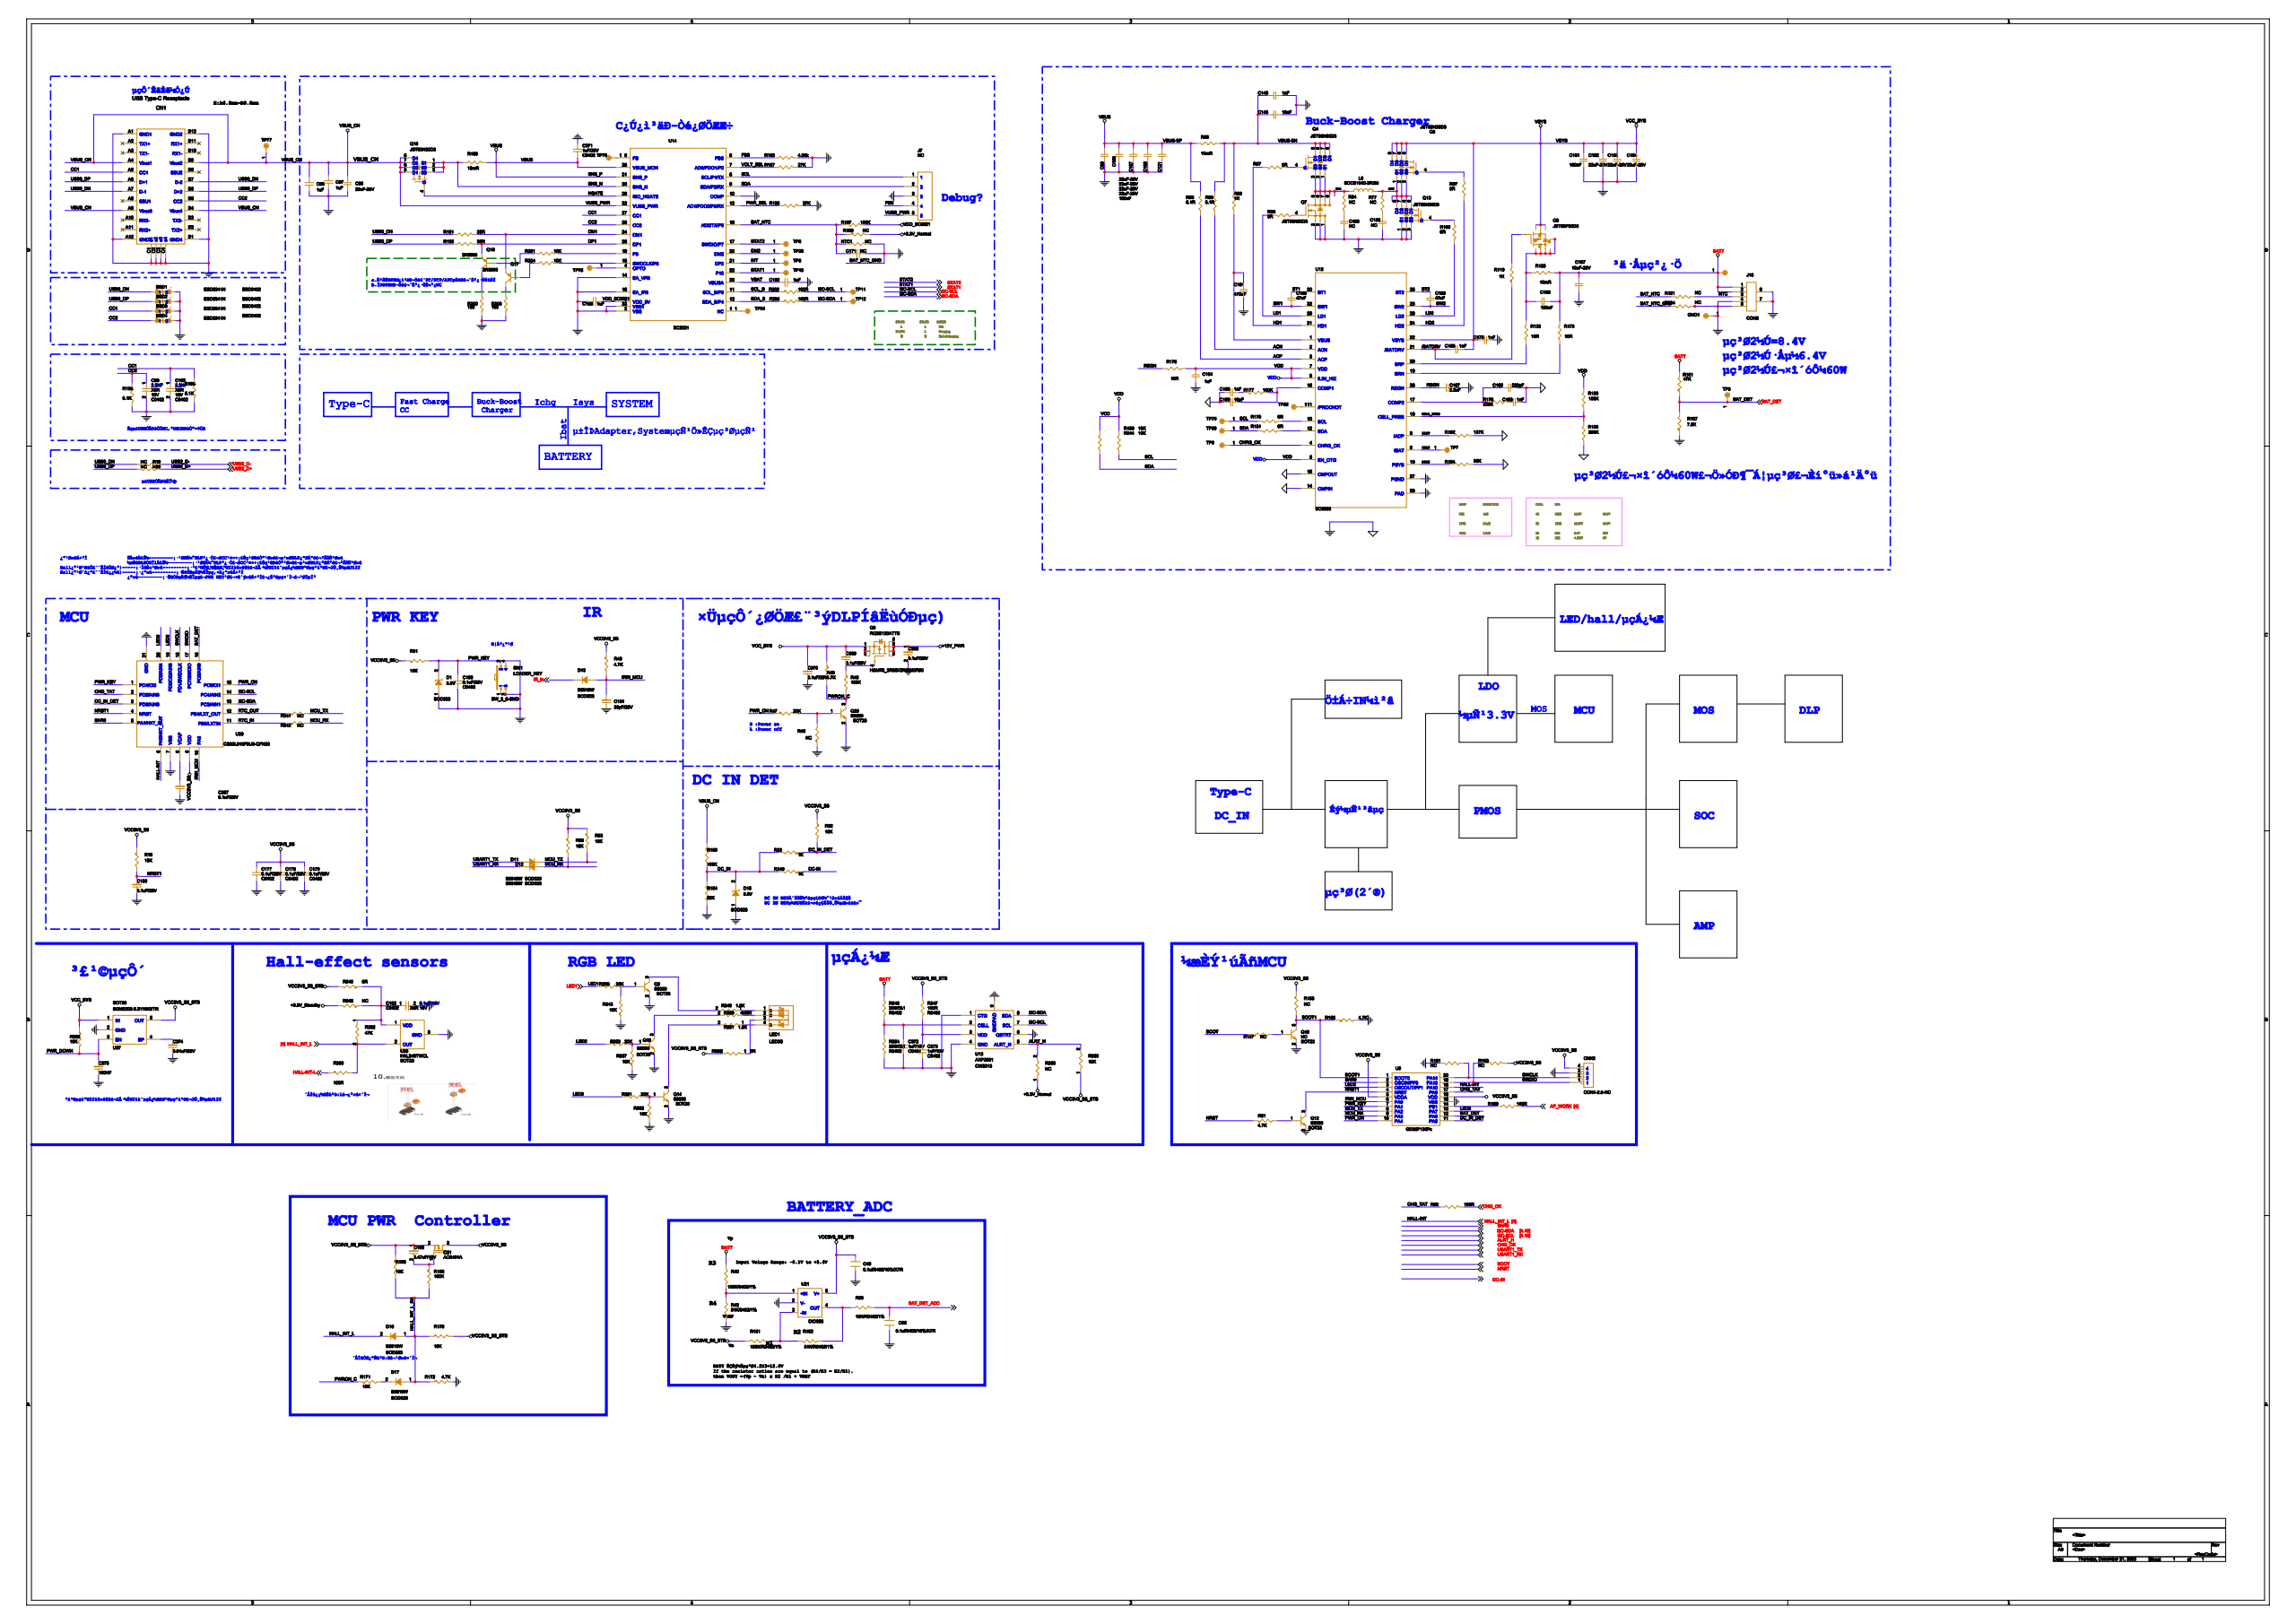Circuit board | Cadence Allegro | 1223 parts | 777 nets | one sheet of the schematic
Parts on this sheet (reference | value | footprint):
C49 | 0.1uf/0402/10%/X7R | C0402
C85 | 0.1uf/0402/10%/X7R | C0402
C95 | 22uF-25V | C1206
C96 | 22uF-25V | C1206
C97 | 1uF | C0402
C98 | 1uF | C0402
C99 | 2.2NF | C0402
C102 | 2.2NF | C0402
C108 | 22uF-25V | C1206
C121 | 100nF | C0402
C148 | 10nF | C0402
C149 | 1nF | C0402
C150 | 22uF-25V | C1206
C151 | 100nF | C0402
C152 | 22uF-25V | C1206
C153 | 22uF-25V | C1206
C154 | 22uF-25V | C1206
C155 | NC | C0402
C156 | NC | C0402
C157 | 10uF-25V | C0805
C158 | 47nF | C0402
C159 | 47nF | C0402
C160 | 100nF | C0402
C161 | 470nF | C0402
C162 | 0.1uF/16V | C0402
C163 | 1nF | C0402
C164 | 1uF | C0402
C165 | 220pF | C0402
C166 | 1nF | C0402
C167 | 2.2uF | C0402
C168 | 1nF | C0402
C169 | 10pF | C0402
C171 | NC | C0402
C175 | 1uF | C0402
C177 | 0.1uF/25V | C0402
C178 | 0.1uF/25V | C0402
C179 | 0.1uF/25V | C0402
C180 | 0.1uF/25V | C0402
C181 | 33pF/25V | C0402
C192 | 1uF | C0402
C193 | 1uF | C0402
C195 | 0.47uF/16V | C0402
C196 | 0.1uF/25V | C0402
C367 | 0.1uF/25V | C0402
C368 | 0.1uF/25V | C0402
C369 | 0.1uF/25V | C0402
C370 | 0.1uF/25V | C0402
C371 | 1uF/25V | C0402
C372 | 1uF/10V | C0402
C373 | 1uF/10V | C0402
C374 | 0.01uF/25V | C0402
C375 | 100NF | C0402
CN1 | USB Type-C Receptacle | USB_TYPE_C
CNX2 | CON4-2.0-NC | DIP4PIN-2P0MM
D1 | 3.3V | SOD323
D11 | B5819W | SOD323
D12 | B5819W | SOD323
D13 | B5819W | SOD323
D15 | 3.3V | SOD323
D16 | B5819W | SOD323
D17 | B5819W | SOD323
ESD1 | ESD5341N | ESD0402
ESD2 | ESD5341N | ESD0402
ESD3 | ESD5341N | ESD0402
ESD4 | ESD5341N | ESD0402
GND2 | DEO | TP06MM
J7 | NC | SIP5P
J10 | CON5 | CN1X5-1P25MM-WF
L6 | SCCB1040-2R2M | L1040
LED1 | LED3S | DIP4PIN-1P25MM
NTC1 | NC | R0603
Q3 | RQ3E120ATTB | HSMT8_3R30X3R30X0R90
Q4 | JST60N30D3 | HSMT8_3R30X3R30X0R90
Q5 | JST60P30D5 | DFN8
Q6 | JST60N30D3 | HSMT8_3R30X3R30X0R90
Q7 | JST60N30D3 | HSMT8_3R30X3R30X0R90
Q9 | S8050 | SOT23
Q10 | S8050 | SOT23
Q12 | S8050 | SOT23
Q13 | JST60N30D3 | HSMT8_3R30X3R30X0R90
Q14 | S8050 | SOT23
Q15 | JST60N30D3 | HSMT8_3R30X3R30X0R90
Q16 | 2N3906 | SOT-23
Q17 | 2N3906 | SOT-23
Q18 | NC | SOT23
Q21 | AO3401A | SOT23-100
Q23 | S8050 | SOT23
R18 | 10K | R0402
R19 | NC | R0402
R20 | NC | R0402
R31 | 10K | R0402
R32 | 10K | R0402
R33 | 1K | R0402
R40 | 100K/0402/1% | R0402
R42 | 51K/0402/1% | R0402
R43 | 4.7K | R0402
R46 | 100K | R0402
R47 | 20K | R0402
R48 | NC | R0402
R49 | 4.7K | R0402
R50 | 100R | R0402
R51 | 4.7K | R0402
R53 | 10K | R0402
R56 | 10mR | R2010
R57 | 0R | R0402
R58 | 5.1R | R0402
R60 | 5.1R | R0402
R63 | 1R | R0402
R64 | NC | R0603
R77 | NC | R0603
R96 | 0R | R0402
R97 | 0R | R0402
R98 | 10K | R0402
R99 | 10K/R0402/1% | R0402
R100 | 0R | R0402
R101 | 47K | R0402
R107 | 7.5K | R0402
R119 | 1K | R0402
R120 | 10mR | R2010
R121 | NC | R0402
R122 | 10R | R0402
R149 | 1K | R0402
R150 | 100K | R0402
R152 | 51K/R0402/1% | R0402
R154 | 22K | R0402
R155 | NC | R0402
R156 | 4.7K | R0402
R157 | NC | R0402
R161 | NC | R0402
R163 | NC | R0402
R166 | 10K | R0402
R167 | 100K | R0402
R168 | 100K | R0402
R169 | 100R | R0402
R170 | 10K | R0402
R171 | 10K | R0402
R172 | 4.7K | R0402
R175 | 10R | R0402
R176 | 10R | R0603
R177 | 100K | R0402
R178 | 330K | R0402
R179 | 0R | R0402
R180 | 100K | R0402
R181 | 0R | R0402
R182 | 137K | R0402
R183 | 300K | R0402
R184 | 30K | R0402
R185 | 4.99k | R0402
R186 | 10mR | R2010
R187 | 27K | R0402
R188 | 27K | R0402
R189 | NC | R0402
R190 | 10K | R0603
R191 | 33R | R0402
R192 | 33R | R0402
R195 | 5.1K | R0402
R196 | 5.1K | R0402
R200 | 100 | R0402
R201 | 10K | R0402
R202 | 100R | R0402
R203 | 100 | R0402
R204 | 10K | R0402
R205 | 100R | R0402
R339 | 20K | R0402
R340 | 0R | R0402
R341 | NC | R0402
R342 | NC | R0402
R344 | 10K | R0603
R345 | 10K | R0402
R346 | 200K%1 | R0402
R347 | 100R | R0402
R348 | NC | R0402
R349 | 1.8K | R0402
R350 | 4.02K | R0402
R351 | 1.8K | R0402
R352 | 47K | R0402
R353 | 20K | R0402
R354 | 200K%1 | R0402
R355 | 10K | R0402
R357 | 10K | R0402
R358 | NC | R0402
R359 | 10K | R0402
R360 | 100R | R0402
R361 | 20K | R0402
R362 | 10K | R0402
R384 | NC | R0402
SW1 | LOADER_KEY | SW_3_6-SMD
TP5 | DEO | TP06MM
TP6 | DEO | TP06MM
TP7 | DEO | TP06MM
TP8 | DEO | TP06MM
TP9 | DEO | TP06MM
TP10 | DEO | TP06MM
TP11 | DEO | TP06MM
TP12 | DEO | TP06MM
TP26 | DEO | TP06MM
TP76 | DEO | TP06MM
TP77 | DEO | TP06MM
TP78 | DEO | TP06MM
TP79 | DEO | TP06MM
TP80 | DEO | TP06MM
TP81 | DEO | TP06MM
TP82 | DEO | TP06MM
U9 | GD32F130Fx | TSSOP20
U12 | SC8886 | QFN32_5X5MM
U13 | AXP2601 | CW2013
U14 | SC2021 | QFN32_5X5MM
U21 | DIO358 | SOT25
U37 | SGM2202-3.3YN5G/TR | SOT25
U38 | HAL248TWCL | SOT23
U39 | CS32L010F8U6-QFN20 | QFN20-3X3MM
Nets of these parts (net: part-pin ...):
GND: C49-1 C85-2 C95-2 C96-2 C97-2 C98-2 C99-2 C102-2 C108-2 C121-2 C148-2 C149-2 C150-2 C151-2 C152-2 C153-2 C154-2 C155-2 C156-2 C157-2 C161-1 C162-2 C164-1 C165-1 C166-1 C167-1 C168-1 C169-1 C171-1 C175-2 C177-2 C178-2 C179-2 C180-2 C181-2 C192-1 C193-2 C196-2 C367-2 C368-2 C370-2 C371-1 C372-2 C373-2 C374-2 C375-2 CN1-A1 CN1-A12 CN1-B1 CN1-B12 CN1-C1 CN1-C2 CN1-C3 CN1-C4 CNX2-3 D1-1 D15-1 ESD1-2 ESD2-2 ESD3-2 ESD4-2 J7-3 J10-4 J10-5 J10-6 J10-7 NTC1-2 Q7-1 Q7-2 Q7-3 Q9-2 Q10-2 Q12-2 Q13-1 Q13-2 Q13-3 Q14-2 Q18-2 Q23-2 R42-2 R48-1 R107-1 R154-1 R156-2 R161-1 R172-2 R182-2 R183-1 R184-2 R185-2 R187-2 R188-2 R195-2 R196-2 R200-2 R203-2 R345-1 R354-1 R357-1 R362-1 R384-1 R384-2 SW1-1 SW1-3 SW1-4 U9-15 U13-1 U13-4 U13-6 U13-9 U21-2 U37-2 U38-3 U12-14 U12-15 U12-27 U12-33 U14-2 U14-10 U14-14 U14-16 U14-33 U39-7 U39-21
I2C-SCL: R202-2 TP11-1 U13-7 U39-14
I2C-SDA: R205-2 TP12-1 U13-8 U39-13
+12V_PWR: C368-1 Q3-5 Q3-6 Q3-7 Q3-8
+3.3V_STANDBY: R348-2
CC1: C102-1 CN1-A5 ESD3-1 R195-1 U14-27
CC2: C99-1 CN1-B5 ESD4-1 R196-1 U14-26
VBUS: C96-1 C108-1 C121-1 C150-1 C371-2 R56-2 R58-2 R186-2 U14-28 U14-31
+3.3V_EMMC: R189-2 R358-1
VCC3V3_S5: C177-1 C178-1 C179-1 CNX2-4 Q21-3 R18-1 R31-1 R32-1 R49-1 R53-1 R98-1 R155-1 R163-1 U9-5 U9-16 U39-9
PWR_KEY: C196-1 D1-2 R31-2 SW1-2 U9-7 U39-1
N25848105: C372-1 R346-1 R354-2 U13-2
N25848164: C373-1 R347-1 U13-3
VCC3V3_S5_STB: C49-2 C195-1 Q21-2 R166-1 R170-2 R340-2 R347-2 R359-1 U21-5 U37-5
N25938331: C195-2 Q21-1 R168-1
VBUS-SN: C148-1 C149-1 Q4-5 Q4-6 Q4-7 Q4-8 R56-1 R60-2 R63-2
VBUS_CN: C95-1 C97-1 C98-1 CN1-A4 CN1-A9 CN1-B4 CN1-B9 J7-5 Q15-5 Q15-6 Q15-7 Q15-8 R150-2 TP77-1 U14-32
VCC_SYS: C151-1 C152-1 C153-1 C154-1 C163-1 C175-1 C369-1 C370-1 Q3-1 Q3-2 Q3-3 Q5-1 Q5-2 Q5-3 Q6-5 Q6-6 Q6-7 Q6-8 R43-1 R355-1 U37-1 U12-22
N253215940: C155-1 R64-1
N253216020: C156-1 R77-1
BATT: C157-1 C160-1 GND2-1 J10-1 J10-2 R40-1 R101-2 R120-2 R175-2 R346-2
SW1: C158-1 L6-1 Q4-1 Q4-2 Q4-3 Q7-5 Q7-6 Q7-7 Q7-8 R64-2 U12-32
BT1: C158-2 U12-30
SW2: C159-1 L6-2 Q6-1 Q6-2 Q6-3 Q13-5 Q13-6 Q13-7 Q13-8 R77-2 U12-23
BT2: C159-2 U12-25
N25320800: C160-2 Q5-5 Q5-6 Q5-7 Q5-8 Q5-9 R120-1 R122-2
N25321914: C161-2 R63-1 U12-1
N25847889: C162-1 R340-1 R348-1 R352-1 U38-1
/BATDRV: C163-2 R119-1 U12-21
VDD: C164-2 R176-1 R180-2 R190-2 R344-2 U12-5 U12-6 U12-7
N25322071: C165-2 R178-1 U12-17
N25803644: C166-2 R177-2
REGN: C167-2 R176-2 U12-28
N25322126: C168-2 R178-2
N25322093: C169-2 R177-1 U12-16
BAT_NTC: C171-2 NTC1-1 R121-2 R167-1 R189-1 U14-15
NRST1: C180-1 Q12-3 R18-2 U9-4 U39-4
N25662857: C367-1 U39-8
N25874642: C369-2 Q3-4 R46-1
IRIN_MCU: C181-1 D13-1 R49-2 U9-6 U39-10
VBAT: C192-2 U14-23
VDD_SC2021: C193-1 R167-2 U14-3
PWR_DOWN: C375-1 R355-2 U37-3
N25848419: C374-1 U37-4
BAT_DET_ADC: C85-1 R99-2
USB0_DP: CN1-A6 CN1-B6 ESD2-1 R20-1 R192-1
USB0_DN: CN1-A7 CN1-B7 ESD1-1 R19-1 R191-1
SWDIO: CNX2-1 R163-2 U9-19 U39-17
SWCLK: CNX2-2 R161-2 U9-20 U39-18
DC_IN: D15-2 R33-2 R149-2 R150-1 R154-2
USART1_TX: D11-1
MCU_TX: D11-2 R53-2 R341-2 U9-8
MCU_RX: D12-1 R98-2 R342-2 U9-9
USART1_RX: D12-2
IR_IN: D13-2
HALL_INT_L_EN: D16-1 D17-1 R166-2 R168-2 R170-1 R172-1
HALL_INT_L: D16-2 R352-2 R360-2 U9-18 U38-2 U39-6
N25938248: D17-2 R171-2
STAT1: TP10-1 U14-22
DM2: TP26-1 U14-20
BAT_DET: R101-1 R107-2 TP5-1 U9-12 U39-16
CHRG_OK: TP6-1 U12-4
IBAT: TP7-1 U12-9
N253223085: TP76-1 U14-6
N25783506: TP78-1 U14-4
SCL: J7-1 R179-2 R190-1 TP79-1 U14-8
STAT2: TP8-1 U14-17
SDA: J7-2 R181-2 R344-1 TP80-1 U14-9
N253223080: TP81-1 U14-1
N2532190210: TP82-1 U12-11
INT: TP9-1 U14-21
NTC: J10-3 R121-1
FBS: J7-4 R185-1 U14-5
N25848250: LED1-1 R349-1
N25848246: LED1-2 R350-1
N25848244: LED1-3
N25848248: LED1-4 R351-1
N25848339: Q10-1 R353-2 R357-2
N25848051: Q10-3 R350-2
N25912891: Q12-1 R51-2
N25848349: Q14-1 R361-2 R362-2
N25848055: Q14-3 R351-2
N25874716: Q23-1 R47-2 R48-2
PWRON_C: Q23-3 R43-2 R46-2 R171-1
N25848315: Q9-1 R339-2 R345-2
N25848049: Q9-3 R349-2
N25806006: Q13-4 R100-1
N25797990: Q4-4 R57-1
N25321472: Q6-4 R97-1
NGATE: Q15-4 U14-29
SNS_N: Q15-1 Q15-2 Q15-3 R186-1 U14-30
N25322754: Q16-1 R201-1
N25322773: Q16-3 R200-1
DP1: Q16-2 R192-2 U14-25
N25322787: Q17-1 R204-1
N25322814: Q17-3 R203-1
DM1: Q17-2 R191-2 U14-24
N25910586: Q18-1 R157-2
BOOT1: Q18-3 R155-2 R156-1 U9-1
N25320670: Q5-4 R119-2
N253216291: Q7-4 R96-1
LD2: R100-2 U12-26
DC_IN_DET: R32-2 R33-1 U9-11 U39-3
N25321910: R122-1 U12-20
DC-IN: R149-1
N25944697: R152-2 U21-3
N25944631: R99-1 R152-1 U21-4
BOOT: R157-1
RTC_OUT: R341-1 U39-12
RTC_IN: R342-1 U39-11
NRST: R51-1
AP_WORK: R169-1
N25910669: R169-2 U9-14
CHG_OK: R50-1
CHG_TAT: R50-2 U9-17 U39-2
USB2_D-: R19-2
USB2_D+: R20-2
N25321912: R175-1 U12-19
N25322166: R179-1 U12-13
N25322168: R181-1 U12-12
CELL_PRES: R180-1 R183-2 U12-18
IADP: R182-1 U12-8
PSYS: R184-1 U12-10
VOLT_SEL: R187-1 U14-7
PWR_SEL: R188-1 U14-13
N25322828: R201-2 U14-19
SCL_S: R202-1 U14-11
SDA_S: R205-1 U14-12
N25322873: R204-2 U14-18
SAR0: U9-2 U39-5
LED1: R339-1
LED2: R353-1 U9-3 U39-20
LED3: R361-1 U9-13 U39-19
PWR_ON: R47-1 U9-10 U39-15
ALRT_H: R358-2 R359-2 U13-5
HALL-INT-L: R360-1
N25944661: R40-2 R42-1 U21-1
HD1: R57-2 U12-31
ACP: R58-1 U12-3
ACN: R60-1 U12-2
LD1: R96-2 U12-29
HD2: R97-2 U12-24